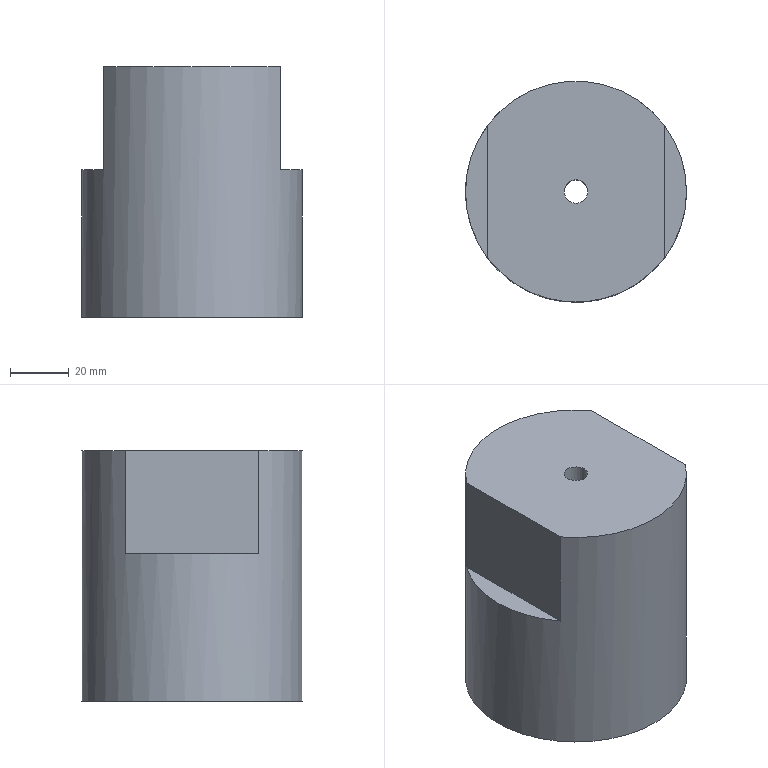Part | NX | features solid 2 | 1 solid | 10 faces | box 75 x 75 x 85 mm | volume 258135 mm3 | plane 7 | cylinder 3 | commonest cylinder face diameters 8 x1 53 x1 75 x1
STEP:
#1=CARTESIAN_POINT('',(-1160.,-557.5,-190.));
#2=VERTEX_POINT('',#1);
#3=CARTESIAN_POINT('',(-1160.,-595.,-190.));
#4=DIRECTION('',(0.,0.,1.));
#5=DIRECTION('',(0.,1.,0.));
#6=AXIS2_PLACEMENT_3D('',#3,#4,#5);
#7=CIRCLE('',#6,37.5);
#8=EDGE_CURVE('',#2,#2,#7,.F.);
#9=ORIENTED_EDGE('',*,*,#8,.F.);
#10=EDGE_LOOP('',(#9));
#11=FACE_BOUND('',#10,.T.);
#12=CARTESIAN_POINT('',(-1130.,-617.5,-105.));
#13=VERTEX_POINT('',#12);
#14=CARTESIAN_POINT('',(-1190.,-617.5,-105.));
#15=VERTEX_POINT('',#14);
#16=CARTESIAN_POINT('',(-1160.,-595.,-105.));
#17=DIRECTION('',(0.,0.,-1.));
#18=DIRECTION('',(1.,0.,0.));
#19=AXIS2_PLACEMENT_3D('',#16,#17,#18);
#20=CIRCLE('',#19,37.5);
#21=EDGE_CURVE('',#13,#15,#20,.T.);
#22=ORIENTED_EDGE('',*,*,#21,.T.);
#23=CARTESIAN_POINT('',(-1190.,-617.5,-140.));
#24=VERTEX_POINT('',#23);
#25=CARTESIAN_POINT('',(-1190.,-617.5,-40.));
#26=DIRECTION('',(0.,0.,-1.));
#27=VECTOR('',#26,1000.);
#28=LINE('',#25,#27);
#29=EDGE_CURVE('',#24,#15,#28,.F.);
#30=ORIENTED_EDGE('',*,*,#29,.F.);
#31=CARTESIAN_POINT('',(-1190.,-572.5,-140.));
#32=VERTEX_POINT('',#31);
#33=CARTESIAN_POINT('',(-1160.,-595.,-140.));
#34=DIRECTION('',(0.,0.,1.));
#35=DIRECTION('',(0.,-1.,0.));
#36=AXIS2_PLACEMENT_3D('',#33,#34,#35);
#37=CIRCLE('',#36,37.5);
#38=EDGE_CURVE('',#32,#24,#37,.T.);
#39=ORIENTED_EDGE('',*,*,#38,.F.);
#40=CARTESIAN_POINT('',(-1190.,-572.5,-105.));
#41=VERTEX_POINT('',#40);
#42=CARTESIAN_POINT('',(-1190.,-572.5,-40.));
#43=DIRECTION('',(0.,0.,-1.));
#44=VECTOR('',#43,1000.);
#45=LINE('',#42,#44);
#46=EDGE_CURVE('',#41,#32,#45,.T.);
#47=ORIENTED_EDGE('',*,*,#46,.F.);
#48=CARTESIAN_POINT('',(-1130.,-572.5,-105.));
#49=VERTEX_POINT('',#48);
#50=CARTESIAN_POINT('',(-1160.,-595.,-105.));
#51=DIRECTION('',(0.,0.,-1.));
#52=DIRECTION('',(1.,0.,0.));
#53=AXIS2_PLACEMENT_3D('',#50,#51,#52);
#54=CIRCLE('',#53,37.5);
#55=EDGE_CURVE('',#41,#49,#54,.T.);
#56=ORIENTED_EDGE('',*,*,#55,.T.);
#57=CARTESIAN_POINT('',(-1130.,-572.5,-140.));
#58=VERTEX_POINT('',#57);
#59=CARTESIAN_POINT('',(-1130.,-572.5,-305.));
#60=DIRECTION('',(0.,0.,1.));
#61=VECTOR('',#60,1000.);
#62=LINE('',#59,#61);
#63=EDGE_CURVE('',#58,#49,#62,.T.);
#64=ORIENTED_EDGE('',*,*,#63,.F.);
#65=CARTESIAN_POINT('',(-1130.,-617.5,-140.));
#66=VERTEX_POINT('',#65);
#67=CARTESIAN_POINT('',(-1160.,-595.,-140.));
#68=DIRECTION('',(0.,0.,-1.));
#69=DIRECTION('',(0.,-1.,0.));
#70=AXIS2_PLACEMENT_3D('',#67,#68,#69);
#71=CIRCLE('',#70,37.5);
#72=EDGE_CURVE('',#58,#66,#71,.T.);
#73=ORIENTED_EDGE('',*,*,#72,.T.);
#74=CARTESIAN_POINT('',(-1130.,-617.5,-305.));
#75=DIRECTION('',(0.,0.,1.));
#76=VECTOR('',#75,1000.);
#77=LINE('',#74,#76);
#78=EDGE_CURVE('',#13,#66,#77,.F.);
#79=ORIENTED_EDGE('',*,*,#78,.F.);
#80=EDGE_LOOP('',(#22,#30,#39,#47,#56,#64,#73,#79));
#81=FACE_BOUND('',#80,.T.);
#82=CARTESIAN_POINT('',(-1160.,-595.,-305.));
#83=DIRECTION('',(0.,0.,1.));
#84=DIRECTION('',(1.,0.,0.));
#85=AXIS2_PLACEMENT_3D('',#82,#83,#84);
#86=CYLINDRICAL_SURFACE('',#85,37.5);
#87=ADVANCED_FACE('',(#11,#81),#86,.T.);
#88=CARTESIAN_POINT('',(-1164.,-595.,-105.));
#89=VERTEX_POINT('',#88);
#90=CARTESIAN_POINT('',(-1160.,-595.,-105.));
#91=DIRECTION('',(0.,0.,1.));
#92=DIRECTION('',(-1.,0.,0.));
#93=AXIS2_PLACEMENT_3D('',#90,#91,#92);
#94=CIRCLE('',#93,4.);
#95=EDGE_CURVE('',#89,#89,#94,.T.);
#96=ORIENTED_EDGE('',*,*,#95,.F.);
#97=EDGE_LOOP('',(#96));
#98=FACE_BOUND('',#97,.T.);
#99=ORIENTED_EDGE('',*,*,#55,.F.);
#100=CARTESIAN_POINT('',(-1190.,-595.,-105.));
#101=DIRECTION('',(0.,-1.,0.));
#102=VECTOR('',#101,1000.);
#103=LINE('',#100,#102);
#104=EDGE_CURVE('',#41,#15,#103,.T.);
#105=ORIENTED_EDGE('',*,*,#104,.T.);
#106=ORIENTED_EDGE('',*,*,#21,.F.);
#107=CARTESIAN_POINT('',(-1130.,-555.,-105.));
#108=DIRECTION('',(0.,-1.,0.));
#109=VECTOR('',#108,1000.);
#110=LINE('',#107,#109);
#111=EDGE_CURVE('',#49,#13,#110,.T.);
#112=ORIENTED_EDGE('',*,*,#111,.F.);
#113=EDGE_LOOP('',(#99,#105,#106,#112));
#114=FACE_BOUND('',#113,.T.);
#115=CARTESIAN_POINT('',(-1160.,-595.,-105.));
#116=DIRECTION('',(0.,0.,1.));
#117=DIRECTION('',(1.,0.,0.));
#118=AXIS2_PLACEMENT_3D('',#115,#116,#117);
#119=PLANE('',#118);
#120=ADVANCED_FACE('',(#98,#114),#119,.T.);
#121=CARTESIAN_POINT('',(-1160.,-568.5,-190.));
#122=VERTEX_POINT('',#121);
#123=CARTESIAN_POINT('',(-1160.,-595.,-190.));
#124=DIRECTION('',(0.,0.,1.));
#125=DIRECTION('',(0.,1.,0.));
#126=AXIS2_PLACEMENT_3D('',#123,#124,#125);
#127=CIRCLE('',#126,26.5);
#128=EDGE_CURVE('',#122,#122,#127,.F.);
#129=ORIENTED_EDGE('',*,*,#128,.F.);
#130=EDGE_LOOP('',(#129));
#131=FACE_BOUND('',#130,.T.);
#132=ORIENTED_EDGE('',*,*,#8,.T.);
#133=EDGE_LOOP('',(#132));
#134=FACE_BOUND('',#133,.T.);
#135=CARTESIAN_POINT('',(-1160.,-595.,-190.));
#136=DIRECTION('',(0.,0.,1.));
#137=DIRECTION('',(1.,0.,0.));
#138=AXIS2_PLACEMENT_3D('',#135,#136,#137);
#139=PLANE('',#138);
#140=ADVANCED_FACE('',(#131,#134),#139,.F.);
#141=ORIENTED_EDGE('',*,*,#111,.T.);
#142=ORIENTED_EDGE('',*,*,#78,.T.);
#143=CARTESIAN_POINT('',(-1130.,-555.,-140.));
#144=DIRECTION('',(0.,-1.,0.));
#145=VECTOR('',#144,1000.);
#146=LINE('',#143,#145);
#147=EDGE_CURVE('',#58,#66,#146,.T.);
#148=ORIENTED_EDGE('',*,*,#147,.F.);
#149=ORIENTED_EDGE('',*,*,#63,.T.);
#150=EDGE_LOOP('',(#141,#142,#148,#149));
#151=FACE_BOUND('',#150,.T.);
#152=CARTESIAN_POINT('',(-1130.,-555.,-230.));
#153=DIRECTION('',(1.,0.,0.));
#154=DIRECTION('',(0.,-1.,0.));
#155=AXIS2_PLACEMENT_3D('',#152,#153,#154);
#156=PLANE('',#155);
#157=ADVANCED_FACE('',(#151),#156,.T.);
#158=ORIENTED_EDGE('',*,*,#72,.F.);
#159=ORIENTED_EDGE('',*,*,#147,.T.);
#160=EDGE_LOOP('',(#158,#159));
#161=FACE_BOUND('',#160,.T.);
#162=CARTESIAN_POINT('',(-1130.,-555.,-140.));
#163=DIRECTION('',(0.,0.,-1.));
#164=DIRECTION('',(-1.,0.,0.));
#165=AXIS2_PLACEMENT_3D('',#162,#163,#164);
#166=PLANE('',#165);
#167=ADVANCED_FACE('',(#161),#166,.F.);
#168=CARTESIAN_POINT('',(-1133.5,-595.,-145.));
#169=VERTEX_POINT('',#168);
#170=CARTESIAN_POINT('',(-1160.,-595.,-145.));
#171=DIRECTION('',(0.,0.,-1.));
#172=DIRECTION('',(1.,0.,0.));
#173=AXIS2_PLACEMENT_3D('',#170,#171,#172);
#174=CIRCLE('',#173,26.5);
#175=EDGE_CURVE('',#169,#169,#174,.T.);
#176=ORIENTED_EDGE('',*,*,#175,.F.);
#177=EDGE_LOOP('',(#176));
#178=FACE_BOUND('',#177,.T.);
#179=ORIENTED_EDGE('',*,*,#128,.T.);
#180=EDGE_LOOP('',(#179));
#181=FACE_BOUND('',#180,.T.);
#182=CARTESIAN_POINT('',(-1160.,-595.,-425.));
#183=DIRECTION('',(0.,0.,1.));
#184=DIRECTION('',(1.,0.,0.));
#185=AXIS2_PLACEMENT_3D('',#182,#183,#184);
#186=CYLINDRICAL_SURFACE('',#185,26.5);
#187=ADVANCED_FACE('',(#178,#181),#186,.F.);
#188=CARTESIAN_POINT('',(-1156.,-595.,-145.));
#189=VERTEX_POINT('',#188);
#190=CARTESIAN_POINT('',(-1160.,-595.,-145.));
#191=DIRECTION('',(0.,0.,-1.));
#192=DIRECTION('',(1.,0.,0.));
#193=AXIS2_PLACEMENT_3D('',#190,#191,#192);
#194=CIRCLE('',#193,4.);
#195=EDGE_CURVE('',#189,#189,#194,.T.);
#196=ORIENTED_EDGE('',*,*,#195,.F.);
#197=EDGE_LOOP('',(#196));
#198=FACE_BOUND('',#197,.T.);
#199=ORIENTED_EDGE('',*,*,#175,.T.);
#200=EDGE_LOOP('',(#199));
#201=FACE_BOUND('',#200,.T.);
#202=CARTESIAN_POINT('',(-1160.,-595.,-145.));
#203=DIRECTION('',(0.,0.,1.));
#204=DIRECTION('',(1.,0.,0.));
#205=AXIS2_PLACEMENT_3D('',#202,#203,#204);
#206=PLANE('',#205);
#207=ADVANCED_FACE('',(#198,#201),#206,.F.);
#208=ORIENTED_EDGE('',*,*,#95,.T.);
#209=EDGE_LOOP('',(#208));
#210=FACE_BOUND('',#209,.T.);
#211=ORIENTED_EDGE('',*,*,#195,.T.);
#212=EDGE_LOOP('',(#211));
#213=FACE_BOUND('',#212,.T.);
#214=CARTESIAN_POINT('',(-1160.,-595.,-105.));
#215=DIRECTION('',(0.,0.,-1.));
#216=DIRECTION('',(-1.,0.,0.));
#217=AXIS2_PLACEMENT_3D('',#214,#215,#216);
#218=CYLINDRICAL_SURFACE('',#217,4.);
#219=ADVANCED_FACE('',(#210,#213),#218,.F.);
#220=ORIENTED_EDGE('',*,*,#46,.T.);
#221=CARTESIAN_POINT('',(-1190.,-555.,-140.));
#222=DIRECTION('',(0.,-1.,0.));
#223=VECTOR('',#222,1000.);
#224=LINE('',#221,#223);
#225=EDGE_CURVE('',#32,#24,#224,.T.);
#226=ORIENTED_EDGE('',*,*,#225,.T.);
#227=ORIENTED_EDGE('',*,*,#29,.T.);
#228=ORIENTED_EDGE('',*,*,#104,.F.);
#229=EDGE_LOOP('',(#220,#226,#227,#228));
#230=FACE_BOUND('',#229,.T.);
#231=CARTESIAN_POINT('',(-1190.,-555.,-40.));
#232=DIRECTION('',(-1.,0.,0.));
#233=DIRECTION('',(0.,1.,0.));
#234=AXIS2_PLACEMENT_3D('',#231,#232,#233);
#235=PLANE('',#234);
#236=ADVANCED_FACE('',(#230),#235,.T.);
#237=ORIENTED_EDGE('',*,*,#38,.T.);
#238=ORIENTED_EDGE('',*,*,#225,.F.);
#239=EDGE_LOOP('',(#237,#238));
#240=FACE_BOUND('',#239,.T.);
#241=CARTESIAN_POINT('',(-1190.,-555.,-140.));
#242=DIRECTION('',(0.,0.,-1.));
#243=DIRECTION('',(1.,0.,0.));
#244=AXIS2_PLACEMENT_3D('',#241,#242,#243);
#245=PLANE('',#244);
#246=ADVANCED_FACE('',(#240),#245,.F.);
#247=CLOSED_SHELL('',(#87,#120,#140,#157,#167,#187,#207,#219,#236,#246));
#248=MANIFOLD_SOLID_BREP('',#247);
#249=(LENGTH_UNIT()NAMED_UNIT(*)SI_UNIT(.MILLI.,.METRE.));
#250=UNCERTAINTY_MEASURE_WITH_UNIT(LENGTH_MEASURE(0.00001),#249,'','');
#251=(NAMED_UNIT(*)PLANE_ANGLE_UNIT()SI_UNIT($,.RADIAN.));
#252=(NAMED_UNIT(*)SI_UNIT($,.STERADIAN.)SOLID_ANGLE_UNIT());
#253=(GEOMETRIC_REPRESENTATION_CONTEXT(3)GLOBAL_UNCERTAINTY_ASSIGNED_CONTEXT((#250))GLOBAL_UNIT_ASSIGNED_CONTEXT((#249,#251,#252))REPRESENTATION_CONTEXT('',''));
#254=ADVANCED_BREP_SHAPE_REPRESENTATION('',(#248),#253);